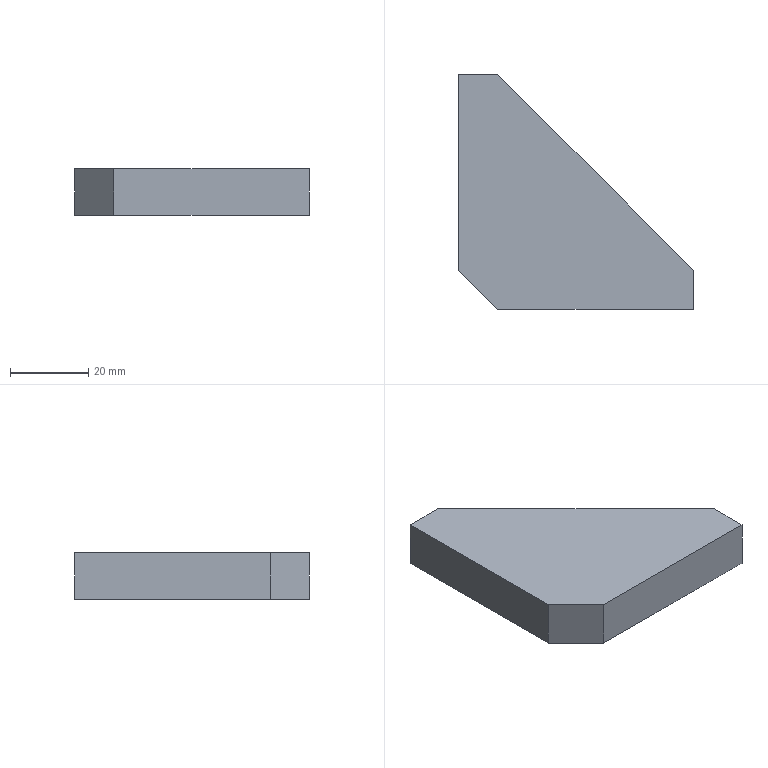Part | STEP file | Rib 9 | 1 solid | 8 faces | box 60 x 60 x 12 mm | volume 27600 mm3 | plane 8
STEP:
#1=CARTESIAN_POINT('',(0.,0.,0.));
#2=DIRECTION('',(0.,0.,1.));
#3=DIRECTION('',(1.,0.,0.));
#4=AXIS2_PLACEMENT_3D('',#1,#2,#3);
#5=CARTESIAN_POINT('',(-1277.,220.,0.));
#6=VERTEX_POINT('',#5);
#7=CARTESIAN_POINT('',(-1277.,170.,0.));
#8=VERTEX_POINT('',#7);
#9=CARTESIAN_POINT('',(-1277.,170.,0.));
#10=DIRECTION('',(0.,-1.,0.));
#11=VECTOR('',#10,1.);
#12=LINE('',#9,#11);
#13=CARTESIAN_POINT('',(-1277.,170.,12.));
#14=DIRECTION('',(1.,0.,0.));
#15=DIRECTION('',(0.,0.,-1.));
#16=AXIS2_PLACEMENT_3D('',#13,#14,#15);
#17=PLANE('',#16);
#18=CARTESIAN_POINT('',(12.,0.));
#19=DIRECTION('',(0.,-1.));
#20=VECTOR('',#19,1.);
#21=LINE('',#18,#20);
#22=(GEOMETRIC_REPRESENTATION_CONTEXT(2)PARAMETRIC_REPRESENTATION_CONTEXT()REPRESENTATION_CONTEXT('',''));
#23=DEFINITIONAL_REPRESENTATION('',(#21),#22);
#24=PCURVE('',#17,#23);
#25=CARTESIAN_POINT('',(-1277.,220.,0.));
#26=DIRECTION('',(0.,0.,-1.));
#27=DIRECTION('',(-1.,0.,0.));
#28=AXIS2_PLACEMENT_3D('',#25,#26,#27);
#29=PLANE('',#28);
#30=CARTESIAN_POINT('',(0.,-50.));
#31=DIRECTION('',(0.,-1.));
#32=VECTOR('',#31,1.);
#33=LINE('',#30,#32);
#34=(GEOMETRIC_REPRESENTATION_CONTEXT(2)PARAMETRIC_REPRESENTATION_CONTEXT()REPRESENTATION_CONTEXT('',''));
#35=DEFINITIONAL_REPRESENTATION('',(#33),#34);
#36=PCURVE('',#29,#35);
#37=SURFACE_CURVE('',#12,(#24,#36),.PCURVE_S1.);
#38=EDGE_CURVE('',#6,#8,#37,.T.);
#39=ORIENTED_EDGE('',*,*,#38,.T.);
#40=CARTESIAN_POINT('',(-1277.,170.,12.));
#41=VERTEX_POINT('',#40);
#42=CARTESIAN_POINT('',(-1277.,170.,12.));
#43=DIRECTION('',(0.,0.,-1.));
#44=VECTOR('',#43,1.);
#45=LINE('',#42,#44);
#46=CARTESIAN_POINT('',(0.,0.));
#47=DIRECTION('',(1.,0.));
#48=VECTOR('',#47,1.);
#49=LINE('',#46,#48);
#50=(GEOMETRIC_REPRESENTATION_CONTEXT(2)PARAMETRIC_REPRESENTATION_CONTEXT()REPRESENTATION_CONTEXT('',''));
#51=DEFINITIONAL_REPRESENTATION('',(#49),#50);
#52=PCURVE('',#17,#51);
#53=CARTESIAN_POINT('',(-1267.,160.,12.));
#54=DIRECTION('',(0.7071,0.7071,0.));
#55=DIRECTION('',(-0.7071,0.7071,0.));
#56=AXIS2_PLACEMENT_3D('',#53,#54,#55);
#57=PLANE('',#56);
#58=CARTESIAN_POINT('',(14.142,0.));
#59=DIRECTION('',(0.,-1.));
#60=VECTOR('',#59,1.);
#61=LINE('',#58,#60);
#62=(GEOMETRIC_REPRESENTATION_CONTEXT(2)PARAMETRIC_REPRESENTATION_CONTEXT()REPRESENTATION_CONTEXT('',''));
#63=DEFINITIONAL_REPRESENTATION('',(#61),#62);
#64=PCURVE('',#57,#63);
#65=SURFACE_CURVE('',#45,(#52,#64),.PCURVE_S1.);
#66=EDGE_CURVE('',#41,#8,#65,.T.);
#67=ORIENTED_EDGE('',*,*,#66,.F.);
#68=CARTESIAN_POINT('',(-1277.,220.,12.));
#69=VERTEX_POINT('',#68);
#70=CARTESIAN_POINT('',(-1277.,170.,12.));
#71=DIRECTION('',(0.,-1.,0.));
#72=VECTOR('',#71,1.);
#73=LINE('',#70,#72);
#74=CARTESIAN_POINT('',(0.,0.));
#75=DIRECTION('',(0.,-1.));
#76=VECTOR('',#75,1.);
#77=LINE('',#74,#76);
#78=(GEOMETRIC_REPRESENTATION_CONTEXT(2)PARAMETRIC_REPRESENTATION_CONTEXT()REPRESENTATION_CONTEXT('',''));
#79=DEFINITIONAL_REPRESENTATION('',(#77),#78);
#80=PCURVE('',#17,#79);
#81=CARTESIAN_POINT('',(-1277.,220.,12.));
#82=DIRECTION('',(0.,0.,-1.));
#83=DIRECTION('',(-1.,0.,0.));
#84=AXIS2_PLACEMENT_3D('',#81,#82,#83);
#85=PLANE('',#84);
#86=CARTESIAN_POINT('',(0.,-50.));
#87=DIRECTION('',(0.,-1.));
#88=VECTOR('',#87,1.);
#89=LINE('',#86,#88);
#90=(GEOMETRIC_REPRESENTATION_CONTEXT(2)PARAMETRIC_REPRESENTATION_CONTEXT()REPRESENTATION_CONTEXT('',''));
#91=DEFINITIONAL_REPRESENTATION('',(#89),#90);
#92=PCURVE('',#85,#91);
#93=SURFACE_CURVE('',#73,(#80,#92),.PCURVE_S1.);
#94=EDGE_CURVE('',#69,#41,#93,.T.);
#95=ORIENTED_EDGE('',*,*,#94,.F.);
#96=CARTESIAN_POINT('',(-1277.,220.,12.));
#97=DIRECTION('',(0.,0.,-1.));
#98=VECTOR('',#97,1.);
#99=LINE('',#96,#98);
#100=CARTESIAN_POINT('',(0.,50.));
#101=DIRECTION('',(1.,0.));
#102=VECTOR('',#101,1.);
#103=LINE('',#100,#102);
#104=(GEOMETRIC_REPRESENTATION_CONTEXT(2)PARAMETRIC_REPRESENTATION_CONTEXT()REPRESENTATION_CONTEXT('',''));
#105=DEFINITIONAL_REPRESENTATION('',(#103),#104);
#106=PCURVE('',#17,#105);
#107=CARTESIAN_POINT('',(-1277.,220.,12.));
#108=DIRECTION('',(0.,-1.,0.));
#109=DIRECTION('',(0.,0.,-1.));
#110=AXIS2_PLACEMENT_3D('',#107,#108,#109);
#111=PLANE('',#110);
#112=CARTESIAN_POINT('',(0.,0.));
#113=DIRECTION('',(1.,0.));
#114=VECTOR('',#113,1.);
#115=LINE('',#112,#114);
#116=(GEOMETRIC_REPRESENTATION_CONTEXT(2)PARAMETRIC_REPRESENTATION_CONTEXT()REPRESENTATION_CONTEXT('',''));
#117=DEFINITIONAL_REPRESENTATION('',(#115),#116);
#118=PCURVE('',#111,#117);
#119=SURFACE_CURVE('',#99,(#106,#118),.PCURVE_S1.);
#120=EDGE_CURVE('',#69,#6,#119,.T.);
#121=ORIENTED_EDGE('',*,*,#120,.T.);
#122=EDGE_LOOP('',(#39,#67,#95,#121));
#123=FACE_BOUND('',#122,.T.);
#124=ADVANCED_FACE('',(#123),#17,.F.);
#125=CARTESIAN_POINT('',(-1267.,160.,0.));
#126=VERTEX_POINT('',#125);
#127=CARTESIAN_POINT('',(-1267.,160.,0.));
#128=DIRECTION('',(0.7071,-0.7071,0.));
#129=VECTOR('',#128,1.);
#130=LINE('',#127,#129);
#131=CARTESIAN_POINT('',(0.,-12.));
#132=DIRECTION('',(-1.,0.));
#133=VECTOR('',#132,1.);
#134=LINE('',#131,#133);
#135=(GEOMETRIC_REPRESENTATION_CONTEXT(2)PARAMETRIC_REPRESENTATION_CONTEXT()REPRESENTATION_CONTEXT('',''));
#136=DEFINITIONAL_REPRESENTATION('',(#134),#135);
#137=PCURVE('',#57,#136);
#138=CARTESIAN_POINT('',(-10.,-60.));
#139=DIRECTION('',(-0.7071,-0.7071));
#140=VECTOR('',#139,1.);
#141=LINE('',#138,#140);
#142=(GEOMETRIC_REPRESENTATION_CONTEXT(2)PARAMETRIC_REPRESENTATION_CONTEXT()REPRESENTATION_CONTEXT('',''));
#143=DEFINITIONAL_REPRESENTATION('',(#141),#142);
#144=PCURVE('',#29,#143);
#145=SURFACE_CURVE('',#130,(#137,#144),.PCURVE_S1.);
#146=EDGE_CURVE('',#8,#126,#145,.T.);
#147=ORIENTED_EDGE('',*,*,#146,.T.);
#148=CARTESIAN_POINT('',(-1267.,160.,12.));
#149=VERTEX_POINT('',#148);
#150=CARTESIAN_POINT('',(-1267.,160.,12.));
#151=DIRECTION('',(0.,0.,-1.));
#152=VECTOR('',#151,1.);
#153=LINE('',#150,#152);
#154=CARTESIAN_POINT('',(0.,0.));
#155=DIRECTION('',(0.,-1.));
#156=VECTOR('',#155,1.);
#157=LINE('',#154,#156);
#158=(GEOMETRIC_REPRESENTATION_CONTEXT(2)PARAMETRIC_REPRESENTATION_CONTEXT()REPRESENTATION_CONTEXT('',''));
#159=DEFINITIONAL_REPRESENTATION('',(#157),#158);
#160=PCURVE('',#57,#159);
#161=CARTESIAN_POINT('',(-1217.,160.,12.));
#162=DIRECTION('',(0.,1.,0.));
#163=DIRECTION('',(0.,0.,1.));
#164=AXIS2_PLACEMENT_3D('',#161,#162,#163);
#165=PLANE('',#164);
#166=CARTESIAN_POINT('',(0.,-50.));
#167=DIRECTION('',(-1.,0.));
#168=VECTOR('',#167,1.);
#169=LINE('',#166,#168);
#170=(GEOMETRIC_REPRESENTATION_CONTEXT(2)PARAMETRIC_REPRESENTATION_CONTEXT()REPRESENTATION_CONTEXT('',''));
#171=DEFINITIONAL_REPRESENTATION('',(#169),#170);
#172=PCURVE('',#165,#171);
#173=SURFACE_CURVE('',#153,(#160,#172),.PCURVE_S1.);
#174=EDGE_CURVE('',#149,#126,#173,.T.);
#175=ORIENTED_EDGE('',*,*,#174,.F.);
#176=CARTESIAN_POINT('',(-1267.,160.,12.));
#177=DIRECTION('',(0.7071,-0.7071,0.));
#178=VECTOR('',#177,1.);
#179=LINE('',#176,#178);
#180=CARTESIAN_POINT('',(0.,0.));
#181=DIRECTION('',(-1.,0.));
#182=VECTOR('',#181,1.);
#183=LINE('',#180,#182);
#184=(GEOMETRIC_REPRESENTATION_CONTEXT(2)PARAMETRIC_REPRESENTATION_CONTEXT()REPRESENTATION_CONTEXT('',''));
#185=DEFINITIONAL_REPRESENTATION('',(#183),#184);
#186=PCURVE('',#57,#185);
#187=CARTESIAN_POINT('',(-10.,-60.));
#188=DIRECTION('',(-0.7071,-0.7071));
#189=VECTOR('',#188,1.);
#190=LINE('',#187,#189);
#191=(GEOMETRIC_REPRESENTATION_CONTEXT(2)PARAMETRIC_REPRESENTATION_CONTEXT()REPRESENTATION_CONTEXT('',''));
#192=DEFINITIONAL_REPRESENTATION('',(#190),#191);
#193=PCURVE('',#85,#192);
#194=SURFACE_CURVE('',#179,(#186,#193),.PCURVE_S1.);
#195=EDGE_CURVE('',#41,#149,#194,.T.);
#196=ORIENTED_EDGE('',*,*,#195,.F.);
#197=ORIENTED_EDGE('',*,*,#66,.T.);
#198=EDGE_LOOP('',(#147,#175,#196,#197));
#199=FACE_BOUND('',#198,.T.);
#200=ADVANCED_FACE('',(#199),#57,.F.);
#201=CARTESIAN_POINT('',(-1217.,160.,0.));
#202=VERTEX_POINT('',#201);
#203=CARTESIAN_POINT('',(-1217.,160.,0.));
#204=DIRECTION('',(1.,0.,0.));
#205=VECTOR('',#204,1.);
#206=LINE('',#203,#205);
#207=CARTESIAN_POINT('',(-12.,0.));
#208=DIRECTION('',(0.,1.));
#209=VECTOR('',#208,1.);
#210=LINE('',#207,#209);
#211=(GEOMETRIC_REPRESENTATION_CONTEXT(2)PARAMETRIC_REPRESENTATION_CONTEXT()REPRESENTATION_CONTEXT('',''));
#212=DEFINITIONAL_REPRESENTATION('',(#210),#211);
#213=PCURVE('',#165,#212);
#214=CARTESIAN_POINT('',(-60.,-60.));
#215=DIRECTION('',(-1.,0.));
#216=VECTOR('',#215,1.);
#217=LINE('',#214,#216);
#218=(GEOMETRIC_REPRESENTATION_CONTEXT(2)PARAMETRIC_REPRESENTATION_CONTEXT()REPRESENTATION_CONTEXT('',''));
#219=DEFINITIONAL_REPRESENTATION('',(#217),#218);
#220=PCURVE('',#29,#219);
#221=SURFACE_CURVE('',#206,(#213,#220),.PCURVE_S1.);
#222=EDGE_CURVE('',#126,#202,#221,.T.);
#223=ORIENTED_EDGE('',*,*,#222,.T.);
#224=CARTESIAN_POINT('',(-1217.,160.,12.));
#225=VERTEX_POINT('',#224);
#226=CARTESIAN_POINT('',(-1217.,160.,12.));
#227=DIRECTION('',(0.,0.,-1.));
#228=VECTOR('',#227,1.);
#229=LINE('',#226,#228);
#230=CARTESIAN_POINT('',(0.,0.));
#231=DIRECTION('',(-1.,0.));
#232=VECTOR('',#231,1.);
#233=LINE('',#230,#232);
#234=(GEOMETRIC_REPRESENTATION_CONTEXT(2)PARAMETRIC_REPRESENTATION_CONTEXT()REPRESENTATION_CONTEXT('',''));
#235=DEFINITIONAL_REPRESENTATION('',(#233),#234);
#236=PCURVE('',#165,#235);
#237=CARTESIAN_POINT('',(-1217.,170.,12.));
#238=DIRECTION('',(-1.,0.,0.));
#239=DIRECTION('',(0.,0.,1.));
#240=AXIS2_PLACEMENT_3D('',#237,#238,#239);
#241=PLANE('',#240);
#242=CARTESIAN_POINT('',(0.,-10.));
#243=DIRECTION('',(-1.,0.));
#244=VECTOR('',#243,1.);
#245=LINE('',#242,#244);
#246=(GEOMETRIC_REPRESENTATION_CONTEXT(2)PARAMETRIC_REPRESENTATION_CONTEXT()REPRESENTATION_CONTEXT('',''));
#247=DEFINITIONAL_REPRESENTATION('',(#245),#246);
#248=PCURVE('',#241,#247);
#249=SURFACE_CURVE('',#229,(#236,#248),.PCURVE_S1.);
#250=EDGE_CURVE('',#225,#202,#249,.T.);
#251=ORIENTED_EDGE('',*,*,#250,.F.);
#252=CARTESIAN_POINT('',(-1217.,160.,12.));
#253=DIRECTION('',(1.,0.,0.));
#254=VECTOR('',#253,1.);
#255=LINE('',#252,#254);
#256=CARTESIAN_POINT('',(0.,0.));
#257=DIRECTION('',(0.,1.));
#258=VECTOR('',#257,1.);
#259=LINE('',#256,#258);
#260=(GEOMETRIC_REPRESENTATION_CONTEXT(2)PARAMETRIC_REPRESENTATION_CONTEXT()REPRESENTATION_CONTEXT('',''));
#261=DEFINITIONAL_REPRESENTATION('',(#259),#260);
#262=PCURVE('',#165,#261);
#263=CARTESIAN_POINT('',(-60.,-60.));
#264=DIRECTION('',(-1.,0.));
#265=VECTOR('',#264,1.);
#266=LINE('',#263,#265);
#267=(GEOMETRIC_REPRESENTATION_CONTEXT(2)PARAMETRIC_REPRESENTATION_CONTEXT()REPRESENTATION_CONTEXT('',''));
#268=DEFINITIONAL_REPRESENTATION('',(#266),#267);
#269=PCURVE('',#85,#268);
#270=SURFACE_CURVE('',#255,(#262,#269),.PCURVE_S1.);
#271=EDGE_CURVE('',#149,#225,#270,.T.);
#272=ORIENTED_EDGE('',*,*,#271,.F.);
#273=ORIENTED_EDGE('',*,*,#174,.T.);
#274=EDGE_LOOP('',(#223,#251,#272,#273));
#275=FACE_BOUND('',#274,.T.);
#276=ADVANCED_FACE('',(#275),#165,.F.);
#277=CARTESIAN_POINT('',(-1217.,170.,0.));
#278=VERTEX_POINT('',#277);
#279=CARTESIAN_POINT('',(-1217.,170.,0.));
#280=DIRECTION('',(0.,1.,0.));
#281=VECTOR('',#280,1.);
#282=LINE('',#279,#281);
#283=CARTESIAN_POINT('',(-12.,0.));
#284=DIRECTION('',(0.,1.));
#285=VECTOR('',#284,1.);
#286=LINE('',#283,#285);
#287=(GEOMETRIC_REPRESENTATION_CONTEXT(2)PARAMETRIC_REPRESENTATION_CONTEXT()REPRESENTATION_CONTEXT('',''));
#288=DEFINITIONAL_REPRESENTATION('',(#286),#287);
#289=PCURVE('',#241,#288);
#290=CARTESIAN_POINT('',(-60.,-50.));
#291=DIRECTION('',(0.,1.));
#292=VECTOR('',#291,1.);
#293=LINE('',#290,#292);
#294=(GEOMETRIC_REPRESENTATION_CONTEXT(2)PARAMETRIC_REPRESENTATION_CONTEXT()REPRESENTATION_CONTEXT('',''));
#295=DEFINITIONAL_REPRESENTATION('',(#293),#294);
#296=PCURVE('',#29,#295);
#297=SURFACE_CURVE('',#282,(#289,#296),.PCURVE_S1.);
#298=EDGE_CURVE('',#202,#278,#297,.T.);
#299=ORIENTED_EDGE('',*,*,#298,.T.);
#300=CARTESIAN_POINT('',(-1217.,170.,12.));
#301=VERTEX_POINT('',#300);
#302=CARTESIAN_POINT('',(-1217.,170.,12.));
#303=DIRECTION('',(0.,0.,-1.));
#304=VECTOR('',#303,1.);
#305=LINE('',#302,#304);
#306=CARTESIAN_POINT('',(0.,0.));
#307=DIRECTION('',(-1.,0.));
#308=VECTOR('',#307,1.);
#309=LINE('',#306,#308);
#310=(GEOMETRIC_REPRESENTATION_CONTEXT(2)PARAMETRIC_REPRESENTATION_CONTEXT()REPRESENTATION_CONTEXT('',''));
#311=DEFINITIONAL_REPRESENTATION('',(#309),#310);
#312=PCURVE('',#241,#311);
#313=CARTESIAN_POINT('',(-1267.,220.,12.));
#314=DIRECTION('',(-0.7071,-0.7071,0.));
#315=DIRECTION('',(0.7071,-0.7071,0.));
#316=AXIS2_PLACEMENT_3D('',#313,#314,#315);
#317=PLANE('',#316);
#318=CARTESIAN_POINT('',(70.711,0.));
#319=DIRECTION('',(0.,-1.));
#320=VECTOR('',#319,1.);
#321=LINE('',#318,#320);
#322=(GEOMETRIC_REPRESENTATION_CONTEXT(2)PARAMETRIC_REPRESENTATION_CONTEXT()REPRESENTATION_CONTEXT('',''));
#323=DEFINITIONAL_REPRESENTATION('',(#321),#322);
#324=PCURVE('',#317,#323);
#325=SURFACE_CURVE('',#305,(#312,#324),.PCURVE_S1.);
#326=EDGE_CURVE('',#301,#278,#325,.T.);
#327=ORIENTED_EDGE('',*,*,#326,.F.);
#328=CARTESIAN_POINT('',(-1217.,170.,12.));
#329=DIRECTION('',(0.,1.,0.));
#330=VECTOR('',#329,1.);
#331=LINE('',#328,#330);
#332=CARTESIAN_POINT('',(0.,0.));
#333=DIRECTION('',(0.,1.));
#334=VECTOR('',#333,1.);
#335=LINE('',#332,#334);
#336=(GEOMETRIC_REPRESENTATION_CONTEXT(2)PARAMETRIC_REPRESENTATION_CONTEXT()REPRESENTATION_CONTEXT('',''));
#337=DEFINITIONAL_REPRESENTATION('',(#335),#336);
#338=PCURVE('',#241,#337);
#339=CARTESIAN_POINT('',(-60.,-50.));
#340=DIRECTION('',(0.,1.));
#341=VECTOR('',#340,1.);
#342=LINE('',#339,#341);
#343=(GEOMETRIC_REPRESENTATION_CONTEXT(2)PARAMETRIC_REPRESENTATION_CONTEXT()REPRESENTATION_CONTEXT('',''));
#344=DEFINITIONAL_REPRESENTATION('',(#342),#343);
#345=PCURVE('',#85,#344);
#346=SURFACE_CURVE('',#331,(#338,#345),.PCURVE_S1.);
#347=EDGE_CURVE('',#225,#301,#346,.T.);
#348=ORIENTED_EDGE('',*,*,#347,.F.);
#349=ORIENTED_EDGE('',*,*,#250,.T.);
#350=EDGE_LOOP('',(#299,#327,#348,#349));
#351=FACE_BOUND('',#350,.T.);
#352=ADVANCED_FACE('',(#351),#241,.F.);
#353=CARTESIAN_POINT('',(-1267.,220.,0.));
#354=VERTEX_POINT('',#353);
#355=CARTESIAN_POINT('',(-1267.,220.,0.));
#356=DIRECTION('',(-0.7071,0.7071,0.));
#357=VECTOR('',#356,1.);
#358=LINE('',#355,#357);
#359=CARTESIAN_POINT('',(0.,-12.));
#360=DIRECTION('',(-1.,0.));
#361=VECTOR('',#360,1.);
#362=LINE('',#359,#361);
#363=(GEOMETRIC_REPRESENTATION_CONTEXT(2)PARAMETRIC_REPRESENTATION_CONTEXT()REPRESENTATION_CONTEXT('',''));
#364=DEFINITIONAL_REPRESENTATION('',(#362),#363);
#365=PCURVE('',#317,#364);
#366=CARTESIAN_POINT('',(-10.,0.));
#367=DIRECTION('',(0.7071,0.7071));
#368=VECTOR('',#367,1.);
#369=LINE('',#366,#368);
#370=(GEOMETRIC_REPRESENTATION_CONTEXT(2)PARAMETRIC_REPRESENTATION_CONTEXT()REPRESENTATION_CONTEXT('',''));
#371=DEFINITIONAL_REPRESENTATION('',(#369),#370);
#372=PCURVE('',#29,#371);
#373=SURFACE_CURVE('',#358,(#365,#372),.PCURVE_S1.);
#374=EDGE_CURVE('',#278,#354,#373,.T.);
#375=ORIENTED_EDGE('',*,*,#374,.T.);
#376=CARTESIAN_POINT('',(-1267.,220.,12.));
#377=VERTEX_POINT('',#376);
#378=CARTESIAN_POINT('',(-1267.,220.,12.));
#379=DIRECTION('',(0.,0.,-1.));
#380=VECTOR('',#379,1.);
#381=LINE('',#378,#380);
#382=CARTESIAN_POINT('',(0.,0.));
#383=DIRECTION('',(0.,-1.));
#384=VECTOR('',#383,1.);
#385=LINE('',#382,#384);
#386=(GEOMETRIC_REPRESENTATION_CONTEXT(2)PARAMETRIC_REPRESENTATION_CONTEXT()REPRESENTATION_CONTEXT('',''));
#387=DEFINITIONAL_REPRESENTATION('',(#385),#386);
#388=PCURVE('',#317,#387);
#389=CARTESIAN_POINT('',(0.,10.));
#390=DIRECTION('',(1.,0.));
#391=VECTOR('',#390,1.);
#392=LINE('',#389,#391);
#393=(GEOMETRIC_REPRESENTATION_CONTEXT(2)PARAMETRIC_REPRESENTATION_CONTEXT()REPRESENTATION_CONTEXT('',''));
#394=DEFINITIONAL_REPRESENTATION('',(#392),#393);
#395=PCURVE('',#111,#394);
#396=SURFACE_CURVE('',#381,(#388,#395),.PCURVE_S1.);
#397=EDGE_CURVE('',#377,#354,#396,.T.);
#398=ORIENTED_EDGE('',*,*,#397,.F.);
#399=CARTESIAN_POINT('',(-1267.,220.,12.));
#400=DIRECTION('',(-0.7071,0.7071,0.));
#401=VECTOR('',#400,1.);
#402=LINE('',#399,#401);
#403=CARTESIAN_POINT('',(0.,0.));
#404=DIRECTION('',(-1.,0.));
#405=VECTOR('',#404,1.);
#406=LINE('',#403,#405);
#407=(GEOMETRIC_REPRESENTATION_CONTEXT(2)PARAMETRIC_REPRESENTATION_CONTEXT()REPRESENTATION_CONTEXT('',''));
#408=DEFINITIONAL_REPRESENTATION('',(#406),#407);
#409=PCURVE('',#317,#408);
#410=CARTESIAN_POINT('',(-10.,0.));
#411=DIRECTION('',(0.7071,0.7071));
#412=VECTOR('',#411,1.);
#413=LINE('',#410,#412);
#414=(GEOMETRIC_REPRESENTATION_CONTEXT(2)PARAMETRIC_REPRESENTATION_CONTEXT()REPRESENTATION_CONTEXT('',''));
#415=DEFINITIONAL_REPRESENTATION('',(#413),#414);
#416=PCURVE('',#85,#415);
#417=SURFACE_CURVE('',#402,(#409,#416),.PCURVE_S1.);
#418=EDGE_CURVE('',#301,#377,#417,.T.);
#419=ORIENTED_EDGE('',*,*,#418,.F.);
#420=ORIENTED_EDGE('',*,*,#326,.T.);
#421=EDGE_LOOP('',(#375,#398,#419,#420));
#422=FACE_BOUND('',#421,.T.);
#423=ADVANCED_FACE('',(#422),#317,.F.);
#424=CARTESIAN_POINT('',(-1277.,220.,0.));
#425=DIRECTION('',(-1.,0.,0.));
#426=VECTOR('',#425,1.);
#427=LINE('',#424,#426);
#428=CARTESIAN_POINT('',(12.,0.));
#429=DIRECTION('',(0.,-1.));
#430=VECTOR('',#429,1.);
#431=LINE('',#428,#430);
#432=(GEOMETRIC_REPRESENTATION_CONTEXT(2)PARAMETRIC_REPRESENTATION_CONTEXT()REPRESENTATION_CONTEXT('',''));
#433=DEFINITIONAL_REPRESENTATION('',(#431),#432);
#434=PCURVE('',#111,#433);
#435=CARTESIAN_POINT('',(0.,0.));
#436=DIRECTION('',(1.,0.));
#437=VECTOR('',#436,1.);
#438=LINE('',#435,#437);
#439=(GEOMETRIC_REPRESENTATION_CONTEXT(2)PARAMETRIC_REPRESENTATION_CONTEXT()REPRESENTATION_CONTEXT('',''));
#440=DEFINITIONAL_REPRESENTATION('',(#438),#439);
#441=PCURVE('',#29,#440);
#442=SURFACE_CURVE('',#427,(#434,#441),.PCURVE_S1.);
#443=EDGE_CURVE('',#354,#6,#442,.T.);
#444=ORIENTED_EDGE('',*,*,#443,.T.);
#445=ORIENTED_EDGE('',*,*,#120,.F.);
#446=CARTESIAN_POINT('',(-1277.,220.,12.));
#447=DIRECTION('',(-1.,0.,0.));
#448=VECTOR('',#447,1.);
#449=LINE('',#446,#448);
#450=CARTESIAN_POINT('',(0.,0.));
#451=DIRECTION('',(0.,-1.));
#452=VECTOR('',#451,1.);
#453=LINE('',#450,#452);
#454=(GEOMETRIC_REPRESENTATION_CONTEXT(2)PARAMETRIC_REPRESENTATION_CONTEXT()REPRESENTATION_CONTEXT('',''));
#455=DEFINITIONAL_REPRESENTATION('',(#453),#454);
#456=PCURVE('',#111,#455);
#457=CARTESIAN_POINT('',(0.,0.));
#458=DIRECTION('',(1.,0.));
#459=VECTOR('',#458,1.);
#460=LINE('',#457,#459);
#461=(GEOMETRIC_REPRESENTATION_CONTEXT(2)PARAMETRIC_REPRESENTATION_CONTEXT()REPRESENTATION_CONTEXT('',''));
#462=DEFINITIONAL_REPRESENTATION('',(#460),#461);
#463=PCURVE('',#85,#462);
#464=SURFACE_CURVE('',#449,(#456,#463),.PCURVE_S1.);
#465=EDGE_CURVE('',#377,#69,#464,.T.);
#466=ORIENTED_EDGE('',*,*,#465,.F.);
#467=ORIENTED_EDGE('',*,*,#397,.T.);
#468=EDGE_LOOP('',(#444,#445,#466,#467));
#469=FACE_BOUND('',#468,.T.);
#470=ADVANCED_FACE('',(#469),#111,.F.);
#471=ORIENTED_EDGE('',*,*,#94,.T.);
#472=ORIENTED_EDGE('',*,*,#195,.T.);
#473=ORIENTED_EDGE('',*,*,#271,.T.);
#474=ORIENTED_EDGE('',*,*,#347,.T.);
#475=ORIENTED_EDGE('',*,*,#418,.T.);
#476=ORIENTED_EDGE('',*,*,#465,.T.);
#477=EDGE_LOOP('',(#471,#472,#473,#474,#475,#476));
#478=FACE_BOUND('',#477,.T.);
#479=ADVANCED_FACE('',(#478),#85,.F.);
#480=ORIENTED_EDGE('',*,*,#38,.F.);
#481=ORIENTED_EDGE('',*,*,#443,.F.);
#482=ORIENTED_EDGE('',*,*,#374,.F.);
#483=ORIENTED_EDGE('',*,*,#298,.F.);
#484=ORIENTED_EDGE('',*,*,#222,.F.);
#485=ORIENTED_EDGE('',*,*,#146,.F.);
#486=EDGE_LOOP('',(#480,#481,#482,#483,#484,#485));
#487=FACE_BOUND('',#486,.T.);
#488=ADVANCED_FACE('',(#487),#29,.T.);
#489=CLOSED_SHELL('',(#124,#200,#276,#352,#423,#470,#479,#488));
#490=MANIFOLD_SOLID_BREP('',#489);
#491=(LENGTH_UNIT()NAMED_UNIT(*)SI_UNIT(.MILLI.,.METRE.));
#492=UNCERTAINTY_MEASURE_WITH_UNIT(LENGTH_MEASURE(0.0000001),#491,'','');
#493=(NAMED_UNIT(*)PLANE_ANGLE_UNIT()SI_UNIT($,.RADIAN.));
#494=(NAMED_UNIT(*)SI_UNIT($,.STERADIAN.)SOLID_ANGLE_UNIT());
#495=(GEOMETRIC_REPRESENTATION_CONTEXT(3)GLOBAL_UNCERTAINTY_ASSIGNED_CONTEXT((#492))GLOBAL_UNIT_ASSIGNED_CONTEXT((#491,#493,#494))REPRESENTATION_CONTEXT('',''));
#496=ADVANCED_BREP_SHAPE_REPRESENTATION('',(#4,#490),#495);